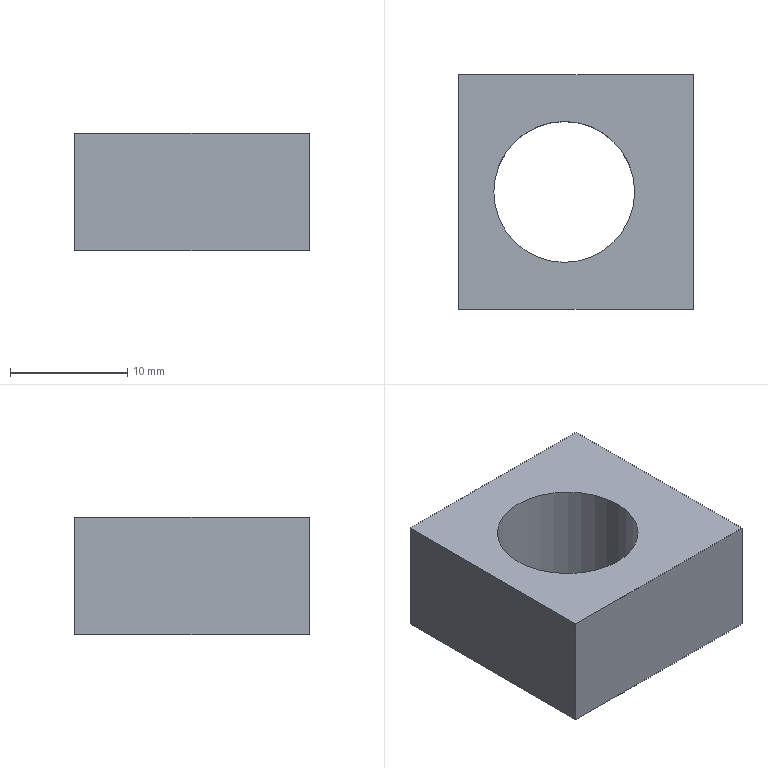Part | SolidWorks | features Extrusion 1 | 1 solid | 8 faces | box 20 x 20 x 10 mm | volume 2869 mm3 | plane 6 | cylinder 2 | commonest cylinder face diameters 12 x2
STEP:
#1=CARTESIAN_POINT('',(-7.,0.,10.));
#2=VERTEX_POINT('',#1);
#3=CARTESIAN_POINT('',(5.,0.,10.));
#4=VERTEX_POINT('',#3);
#5=CARTESIAN_POINT('',(-1.,0.,10.));
#6=DIRECTION('',(0.,0.,1.));
#7=DIRECTION('',(1.,0.,0.));
#8=AXIS2_PLACEMENT_3D('',#5,#6,#7);
#9=CIRCLE('',#8,6.);
#10=EDGE_CURVE('',#2,#4,#9,.T.);
#11=ORIENTED_EDGE('',*,*,#10,.T.);
#12=CARTESIAN_POINT('',(5.,0.,0.));
#13=VERTEX_POINT('',#12);
#14=CARTESIAN_POINT('',(5.,0.,10.));
#15=DIRECTION('',(0.,0.,-1.));
#16=VECTOR('',#15,1000.);
#17=LINE('',#14,#16);
#18=EDGE_CURVE('',#4,#13,#17,.T.);
#19=ORIENTED_EDGE('',*,*,#18,.T.);
#20=CARTESIAN_POINT('',(-7.,0.,0.));
#21=VERTEX_POINT('',#20);
#22=CARTESIAN_POINT('',(-1.,0.,0.));
#23=DIRECTION('',(0.,0.,1.));
#24=DIRECTION('',(1.,0.,0.));
#25=AXIS2_PLACEMENT_3D('',#22,#23,#24);
#26=CIRCLE('',#25,6.);
#27=EDGE_CURVE('',#21,#13,#26,.T.);
#28=ORIENTED_EDGE('',*,*,#27,.F.);
#29=CARTESIAN_POINT('',(-7.,0.,10.));
#30=DIRECTION('',(0.,0.,-1.));
#31=VECTOR('',#30,1000.);
#32=LINE('',#29,#31);
#33=EDGE_CURVE('',#2,#21,#32,.T.);
#34=ORIENTED_EDGE('',*,*,#33,.F.);
#35=EDGE_LOOP('',(#11,#19,#28,#34));
#36=FACE_OUTER_BOUND('',#35,.T.);
#37=CARTESIAN_POINT('',(-1.,0.,10.));
#38=DIRECTION('',(0.,0.,-1.));
#39=DIRECTION('',(-1.,0.,0.));
#40=AXIS2_PLACEMENT_3D('',#37,#38,#39);
#41=CYLINDRICAL_SURFACE('',#40,6.);
#42=ADVANCED_FACE('',(#36),#41,.F.);
#43=CARTESIAN_POINT('',(10.,-10.,10.));
#44=VERTEX_POINT('',#43);
#45=CARTESIAN_POINT('',(10.,10.,10.));
#46=VERTEX_POINT('',#45);
#47=CARTESIAN_POINT('',(10.,10.,10.));
#48=DIRECTION('',(0.,1.,0.));
#49=VECTOR('',#48,1000.);
#50=LINE('',#47,#49);
#51=EDGE_CURVE('',#44,#46,#50,.T.);
#52=ORIENTED_EDGE('',*,*,#51,.T.);
#53=CARTESIAN_POINT('',(-10.,10.,10.));
#54=VERTEX_POINT('',#53);
#55=CARTESIAN_POINT('',(-10.,10.,10.));
#56=DIRECTION('',(-1.,0.,0.));
#57=VECTOR('',#56,1000.);
#58=LINE('',#55,#57);
#59=EDGE_CURVE('',#46,#54,#58,.T.);
#60=ORIENTED_EDGE('',*,*,#59,.T.);
#61=CARTESIAN_POINT('',(-10.,-10.,10.));
#62=VERTEX_POINT('',#61);
#63=CARTESIAN_POINT('',(-10.,10.,10.));
#64=DIRECTION('',(0.,-1.,0.));
#65=VECTOR('',#64,1000.);
#66=LINE('',#63,#65);
#67=EDGE_CURVE('',#54,#62,#66,.T.);
#68=ORIENTED_EDGE('',*,*,#67,.T.);
#69=CARTESIAN_POINT('',(-10.,-10.,10.));
#70=DIRECTION('',(1.,0.,0.));
#71=VECTOR('',#70,1000.);
#72=LINE('',#69,#71);
#73=EDGE_CURVE('',#62,#44,#72,.T.);
#74=ORIENTED_EDGE('',*,*,#73,.T.);
#75=EDGE_LOOP('',(#52,#60,#68,#74));
#76=FACE_OUTER_BOUND('',#75,.T.);
#77=ORIENTED_EDGE('',*,*,#10,.F.);
#78=CARTESIAN_POINT('',(-1.,0.,10.));
#79=DIRECTION('',(0.,0.,1.));
#80=DIRECTION('',(1.,0.,0.));
#81=AXIS2_PLACEMENT_3D('',#78,#79,#80);
#82=CIRCLE('',#81,6.);
#83=EDGE_CURVE('',#4,#2,#82,.T.);
#84=ORIENTED_EDGE('',*,*,#83,.F.);
#85=EDGE_LOOP('',(#77,#84));
#86=FACE_BOUND('',#85,.T.);
#87=CARTESIAN_POINT('',(0.,0.,10.));
#88=DIRECTION('',(0.,0.,1.));
#89=DIRECTION('',(1.,0.,0.));
#90=AXIS2_PLACEMENT_3D('',#87,#88,#89);
#91=PLANE('',#90);
#92=ADVANCED_FACE('',(#76,#86),#91,.T.);
#93=CARTESIAN_POINT('',(10.,-10.,0.));
#94=VERTEX_POINT('',#93);
#95=CARTESIAN_POINT('',(10.,10.,0.));
#96=VERTEX_POINT('',#95);
#97=CARTESIAN_POINT('',(10.,10.,0.));
#98=DIRECTION('',(0.,1.,0.));
#99=VECTOR('',#98,1000.);
#100=LINE('',#97,#99);
#101=EDGE_CURVE('',#94,#96,#100,.T.);
#102=ORIENTED_EDGE('',*,*,#101,.F.);
#103=CARTESIAN_POINT('',(-10.,-10.,0.));
#104=VERTEX_POINT('',#103);
#105=CARTESIAN_POINT('',(-10.,-10.,0.));
#106=DIRECTION('',(1.,0.,0.));
#107=VECTOR('',#106,1000.);
#108=LINE('',#105,#107);
#109=EDGE_CURVE('',#104,#94,#108,.T.);
#110=ORIENTED_EDGE('',*,*,#109,.F.);
#111=CARTESIAN_POINT('',(-10.,10.,0.));
#112=VERTEX_POINT('',#111);
#113=CARTESIAN_POINT('',(-10.,10.,0.));
#114=DIRECTION('',(0.,-1.,0.));
#115=VECTOR('',#114,1000.);
#116=LINE('',#113,#115);
#117=EDGE_CURVE('',#112,#104,#116,.T.);
#118=ORIENTED_EDGE('',*,*,#117,.F.);
#119=CARTESIAN_POINT('',(-10.,10.,0.));
#120=DIRECTION('',(-1.,0.,0.));
#121=VECTOR('',#120,1000.);
#122=LINE('',#119,#121);
#123=EDGE_CURVE('',#96,#112,#122,.T.);
#124=ORIENTED_EDGE('',*,*,#123,.F.);
#125=EDGE_LOOP('',(#102,#110,#118,#124));
#126=FACE_OUTER_BOUND('',#125,.T.);
#127=ORIENTED_EDGE('',*,*,#27,.T.);
#128=CARTESIAN_POINT('',(-1.,0.,0.));
#129=DIRECTION('',(0.,0.,1.));
#130=DIRECTION('',(1.,0.,0.));
#131=AXIS2_PLACEMENT_3D('',#128,#129,#130);
#132=CIRCLE('',#131,6.);
#133=EDGE_CURVE('',#13,#21,#132,.T.);
#134=ORIENTED_EDGE('',*,*,#133,.T.);
#135=EDGE_LOOP('',(#127,#134));
#136=FACE_BOUND('',#135,.T.);
#137=CARTESIAN_POINT('',(0.,0.,0.));
#138=DIRECTION('',(0.,0.,1.));
#139=DIRECTION('',(1.,0.,0.));
#140=AXIS2_PLACEMENT_3D('',#137,#138,#139);
#141=PLANE('',#140);
#142=ADVANCED_FACE('',(#126,#136),#141,.F.);
#143=ORIENTED_EDGE('',*,*,#101,.T.);
#144=CARTESIAN_POINT('',(10.,10.,10.));
#145=DIRECTION('',(0.,0.,-1.));
#146=VECTOR('',#145,1000.);
#147=LINE('',#144,#146);
#148=EDGE_CURVE('',#46,#96,#147,.T.);
#149=ORIENTED_EDGE('',*,*,#148,.F.);
#150=ORIENTED_EDGE('',*,*,#51,.F.);
#151=CARTESIAN_POINT('',(10.,-10.,10.));
#152=DIRECTION('',(0.,0.,-1.));
#153=VECTOR('',#152,1000.);
#154=LINE('',#151,#153);
#155=EDGE_CURVE('',#44,#94,#154,.T.);
#156=ORIENTED_EDGE('',*,*,#155,.T.);
#157=EDGE_LOOP('',(#143,#149,#150,#156));
#158=FACE_OUTER_BOUND('',#157,.T.);
#159=CARTESIAN_POINT('',(10.,10.,10.));
#160=DIRECTION('',(-1.,0.,0.));
#161=DIRECTION('',(0.,-1.,0.));
#162=AXIS2_PLACEMENT_3D('',#159,#160,#161);
#163=PLANE('',#162);
#164=ADVANCED_FACE('',(#158),#163,.F.);
#165=ORIENTED_EDGE('',*,*,#123,.T.);
#166=CARTESIAN_POINT('',(-10.,10.,10.));
#167=DIRECTION('',(0.,0.,-1.));
#168=VECTOR('',#167,1000.);
#169=LINE('',#166,#168);
#170=EDGE_CURVE('',#54,#112,#169,.T.);
#171=ORIENTED_EDGE('',*,*,#170,.F.);
#172=ORIENTED_EDGE('',*,*,#59,.F.);
#173=ORIENTED_EDGE('',*,*,#148,.T.);
#174=EDGE_LOOP('',(#165,#171,#172,#173));
#175=FACE_OUTER_BOUND('',#174,.T.);
#176=CARTESIAN_POINT('',(-10.,10.,10.));
#177=DIRECTION('',(0.,-1.,0.));
#178=DIRECTION('',(0.,0.,-1.));
#179=AXIS2_PLACEMENT_3D('',#176,#177,#178);
#180=PLANE('',#179);
#181=ADVANCED_FACE('',(#175),#180,.F.);
#182=ORIENTED_EDGE('',*,*,#117,.T.);
#183=CARTESIAN_POINT('',(-10.,-10.,10.));
#184=DIRECTION('',(0.,0.,-1.));
#185=VECTOR('',#184,1000.);
#186=LINE('',#183,#185);
#187=EDGE_CURVE('',#62,#104,#186,.T.);
#188=ORIENTED_EDGE('',*,*,#187,.F.);
#189=ORIENTED_EDGE('',*,*,#67,.F.);
#190=ORIENTED_EDGE('',*,*,#170,.T.);
#191=EDGE_LOOP('',(#182,#188,#189,#190));
#192=FACE_OUTER_BOUND('',#191,.T.);
#193=CARTESIAN_POINT('',(-10.,10.,10.));
#194=DIRECTION('',(1.,0.,0.));
#195=DIRECTION('',(0.,1.,0.));
#196=AXIS2_PLACEMENT_3D('',#193,#194,#195);
#197=PLANE('',#196);
#198=ADVANCED_FACE('',(#192),#197,.F.);
#199=ORIENTED_EDGE('',*,*,#109,.T.);
#200=ORIENTED_EDGE('',*,*,#155,.F.);
#201=ORIENTED_EDGE('',*,*,#73,.F.);
#202=ORIENTED_EDGE('',*,*,#187,.T.);
#203=EDGE_LOOP('',(#199,#200,#201,#202));
#204=FACE_OUTER_BOUND('',#203,.T.);
#205=CARTESIAN_POINT('',(-10.,-10.,10.));
#206=DIRECTION('',(0.,1.,0.));
#207=DIRECTION('',(0.,0.,1.));
#208=AXIS2_PLACEMENT_3D('',#205,#206,#207);
#209=PLANE('',#208);
#210=ADVANCED_FACE('',(#204),#209,.F.);
#211=ORIENTED_EDGE('',*,*,#18,.F.);
#212=ORIENTED_EDGE('',*,*,#83,.T.);
#213=ORIENTED_EDGE('',*,*,#33,.T.);
#214=ORIENTED_EDGE('',*,*,#133,.F.);
#215=EDGE_LOOP('',(#211,#212,#213,#214));
#216=FACE_OUTER_BOUND('',#215,.T.);
#217=CARTESIAN_POINT('',(-1.,0.,10.));
#218=DIRECTION('',(0.,0.,-1.));
#219=DIRECTION('',(-1.,0.,0.));
#220=AXIS2_PLACEMENT_3D('',#217,#218,#219);
#221=CYLINDRICAL_SURFACE('',#220,6.);
#222=ADVANCED_FACE('',(#216),#221,.F.);
#223=CLOSED_SHELL('',(#42,#92,#142,#164,#181,#198,#210,#222));
#224=MANIFOLD_SOLID_BREP('',#223);
#225=CARTESIAN_POINT('',(0.,0.,0.));
#226=DIRECTION('',(0.,0.,1.));
#227=DIRECTION('',(1.,0.,0.));
#228=AXIS2_PLACEMENT_3D('',#225,#226,#227);
#229=(LENGTH_UNIT()NAMED_UNIT(*)SI_UNIT(.MILLI.,.METRE.));
#230=UNCERTAINTY_MEASURE_WITH_UNIT(LENGTH_MEASURE(0.00001),#229,'','');
#231=(NAMED_UNIT(*)PLANE_ANGLE_UNIT()SI_UNIT($,.RADIAN.));
#232=(NAMED_UNIT(*)SI_UNIT($,.STERADIAN.)SOLID_ANGLE_UNIT());
#233=(GEOMETRIC_REPRESENTATION_CONTEXT(3)GLOBAL_UNCERTAINTY_ASSIGNED_CONTEXT((#230))GLOBAL_UNIT_ASSIGNED_CONTEXT((#229,#231,#232))REPRESENTATION_CONTEXT('',''));
#234=ADVANCED_BREP_SHAPE_REPRESENTATION('',(#224,#228),#233);